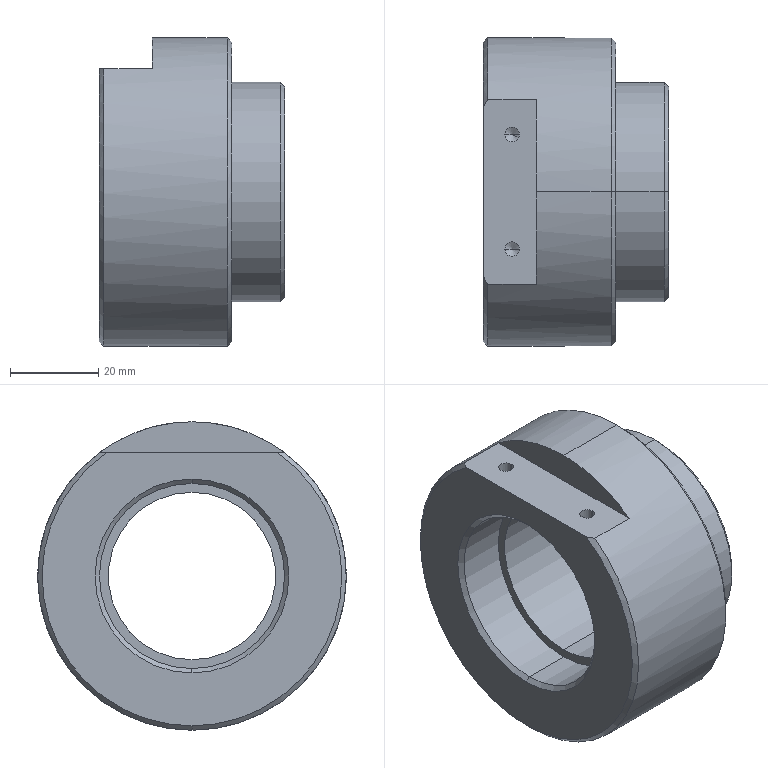Part | SolidWorks | features ICE 5, HoleWzd 2, Chamfer 1, CirPattern 1, Cut 1, Extrusion 1 | 1 solid | 51 faces | box 42 x 70 x 70 mm | volume 81911 mm3 | cone 22 | cylinder 22 | plane 7 | commonest cylinder face diameters 3.3 x12 42 x4 38 x2 49.9 x2 70 x2
STEP:
#1=CARTESIAN_POINT('',(0.,0.,-34.));
#2=VERTEX_POINT('',#1);
#3=CARTESIAN_POINT('',(0.,-19.287,28.));
#4=VERTEX_POINT('',#3);
#5=CARTESIAN_POINT('',(0.,0.,0.));
#6=DIRECTION('',(-1.,0.,0.));
#7=DIRECTION('',(0.,0.,-1.));
#8=AXIS2_PLACEMENT_3D('',#5,#6,#7);
#9=CIRCLE('',#8,34.);
#10=EDGE_CURVE('',#2,#4,#9,.T.);
#11=ORIENTED_EDGE('',*,*,#10,.F.);
#12=CARTESIAN_POINT('',(1.,0.,-35.));
#13=VERTEX_POINT('',#12);
#14=CARTESIAN_POINT('',(1.,0.,-35.));
#15=DIRECTION('',(0.7071,0.,-0.7071));
#16=VECTOR('',#15,1000.);
#17=LINE('',#14,#16);
#18=EDGE_CURVE('',#2,#13,#17,.T.);
#19=ORIENTED_EDGE('',*,*,#18,.T.);
#20=CARTESIAN_POINT('',(1.,-21.,28.));
#21=VERTEX_POINT('',#20);
#22=CARTESIAN_POINT('',(1.,0.,0.));
#23=DIRECTION('',(1.,0.,0.));
#24=DIRECTION('',(0.,0.,-1.));
#25=AXIS2_PLACEMENT_3D('',#22,#23,#24);
#26=CIRCLE('',#25,35.);
#27=EDGE_CURVE('',#21,#13,#26,.T.);
#28=ORIENTED_EDGE('',*,*,#27,.F.);
#29=CARTESIAN_POINT('',(0.,-19.287,28.));
#30=CARTESIAN_POINT('',(0.3262,-19.862,28.));
#31=CARTESIAN_POINT('',(0.6598,-20.433,28.));
#32=CARTESIAN_POINT('',(1.,-21.,28.));
#33=B_SPLINE_CURVE_WITH_KNOTS('',3,(#29,#30,#31,#32),.UNSPECIFIED.,.F.,.F.,(4,4),(0.,0.001983),.UNSPECIFIED.);
#34=EDGE_CURVE('',#4,#21,#33,.T.);
#35=ORIENTED_EDGE('',*,*,#34,.F.);
#36=EDGE_LOOP('',(#11,#19,#28,#35));
#37=FACE_OUTER_BOUND('',#36,.T.);
#38=CARTESIAN_POINT('',(1.,0.,0.));
#39=DIRECTION('',(1.,0.,0.));
#40=DIRECTION('',(0.,0.,-1.));
#41=AXIS2_PLACEMENT_3D('',#38,#39,#40);
#42=CONICAL_SURFACE('',#41,35.,0.7854);
#43=ADVANCED_FACE('',(#37),#42,.T.);
#44=CARTESIAN_POINT('',(30.,0.,-34.));
#45=VERTEX_POINT('',#44);
#46=CARTESIAN_POINT('',(30.,0.,34.));
#47=VERTEX_POINT('',#46);
#48=CARTESIAN_POINT('',(30.,0.,0.));
#49=DIRECTION('',(1.,0.,0.));
#50=DIRECTION('',(0.,0.,-1.));
#51=AXIS2_PLACEMENT_3D('',#48,#49,#50);
#52=CIRCLE('',#51,34.);
#53=EDGE_CURVE('',#45,#47,#52,.T.);
#54=ORIENTED_EDGE('',*,*,#53,.F.);
#55=CARTESIAN_POINT('',(29.,0.,-35.));
#56=VERTEX_POINT('',#55);
#57=CARTESIAN_POINT('',(30.,0.,-34.));
#58=DIRECTION('',(-0.7071,0.,-0.7071));
#59=VECTOR('',#58,1000.);
#60=LINE('',#57,#59);
#61=EDGE_CURVE('',#45,#56,#60,.T.);
#62=ORIENTED_EDGE('',*,*,#61,.T.);
#63=CARTESIAN_POINT('',(29.,0.,35.));
#64=VERTEX_POINT('',#63);
#65=CARTESIAN_POINT('',(29.,0.,0.));
#66=DIRECTION('',(-1.,0.,0.));
#67=DIRECTION('',(0.,0.,-1.));
#68=AXIS2_PLACEMENT_3D('',#65,#66,#67);
#69=CIRCLE('',#68,35.);
#70=EDGE_CURVE('',#64,#56,#69,.T.);
#71=ORIENTED_EDGE('',*,*,#70,.F.);
#72=CARTESIAN_POINT('',(30.,0.,34.));
#73=DIRECTION('',(-0.7071,0.,0.7071));
#74=VECTOR('',#73,1000.);
#75=LINE('',#72,#74);
#76=EDGE_CURVE('',#47,#64,#75,.T.);
#77=ORIENTED_EDGE('',*,*,#76,.F.);
#78=EDGE_LOOP('',(#54,#62,#71,#77));
#79=FACE_OUTER_BOUND('',#78,.T.);
#80=CARTESIAN_POINT('',(30.,0.,0.));
#81=DIRECTION('',(-1.,0.,0.));
#82=DIRECTION('',(0.,0.,1.));
#83=AXIS2_PLACEMENT_3D('',#80,#81,#82);
#84=CONICAL_SURFACE('',#83,34.,0.7854);
#85=ADVANCED_FACE('',(#79),#84,.T.);
#86=CARTESIAN_POINT('',(42.,0.,-23.95));
#87=VERTEX_POINT('',#86);
#88=CARTESIAN_POINT('',(42.,0.,23.95));
#89=VERTEX_POINT('',#88);
#90=CARTESIAN_POINT('',(42.,0.,0.));
#91=DIRECTION('',(1.,0.,0.));
#92=DIRECTION('',(0.,0.,-1.));
#93=AXIS2_PLACEMENT_3D('',#90,#91,#92);
#94=CIRCLE('',#93,23.95);
#95=EDGE_CURVE('',#87,#89,#94,.T.);
#96=ORIENTED_EDGE('',*,*,#95,.F.);
#97=CARTESIAN_POINT('',(41.,0.,-24.95));
#98=VERTEX_POINT('',#97);
#99=CARTESIAN_POINT('',(42.,0.,-23.95));
#100=DIRECTION('',(-0.7071,0.,-0.7071));
#101=VECTOR('',#100,1000.);
#102=LINE('',#99,#101);
#103=EDGE_CURVE('',#87,#98,#102,.T.);
#104=ORIENTED_EDGE('',*,*,#103,.T.);
#105=CARTESIAN_POINT('',(41.,0.,24.95));
#106=VERTEX_POINT('',#105);
#107=CARTESIAN_POINT('',(41.,0.,0.));
#108=DIRECTION('',(-1.,0.,0.));
#109=DIRECTION('',(0.,0.,-1.));
#110=AXIS2_PLACEMENT_3D('',#107,#108,#109);
#111=CIRCLE('',#110,24.95);
#112=EDGE_CURVE('',#106,#98,#111,.T.);
#113=ORIENTED_EDGE('',*,*,#112,.F.);
#114=CARTESIAN_POINT('',(42.,0.,23.95));
#115=DIRECTION('',(-0.7071,0.,0.7071));
#116=VECTOR('',#115,1000.);
#117=LINE('',#114,#116);
#118=EDGE_CURVE('',#89,#106,#117,.T.);
#119=ORIENTED_EDGE('',*,*,#118,.F.);
#120=EDGE_LOOP('',(#96,#104,#113,#119));
#121=FACE_OUTER_BOUND('',#120,.T.);
#122=CARTESIAN_POINT('',(42.,0.,0.));
#123=DIRECTION('',(-1.,0.,0.));
#124=DIRECTION('',(0.,0.,1.));
#125=AXIS2_PLACEMENT_3D('',#122,#123,#124);
#126=CONICAL_SURFACE('',#125,23.95,0.7854);
#127=ADVANCED_FACE('',(#121),#126,.T.);
#128=CARTESIAN_POINT('',(41.,0.,21.));
#129=VERTEX_POINT('',#128);
#130=CARTESIAN_POINT('',(41.,0.,-21.));
#131=VERTEX_POINT('',#130);
#132=CARTESIAN_POINT('',(41.,0.,0.));
#133=DIRECTION('',(1.,0.,0.));
#134=DIRECTION('',(0.,0.,-1.));
#135=AXIS2_PLACEMENT_3D('',#132,#133,#134);
#136=CIRCLE('',#135,21.);
#137=EDGE_CURVE('',#129,#131,#136,.T.);
#138=ORIENTED_EDGE('',*,*,#137,.F.);
#139=CARTESIAN_POINT('',(42.,0.,22.));
#140=VERTEX_POINT('',#139);
#141=CARTESIAN_POINT('',(41.,0.,21.));
#142=DIRECTION('',(0.7071,0.,0.7071));
#143=VECTOR('',#142,1000.);
#144=LINE('',#141,#143);
#145=EDGE_CURVE('',#129,#140,#144,.T.);
#146=ORIENTED_EDGE('',*,*,#145,.T.);
#147=CARTESIAN_POINT('',(42.,0.,-22.));
#148=VERTEX_POINT('',#147);
#149=CARTESIAN_POINT('',(42.,0.,0.));
#150=DIRECTION('',(-1.,0.,0.));
#151=DIRECTION('',(0.,0.,-1.));
#152=AXIS2_PLACEMENT_3D('',#149,#150,#151);
#153=CIRCLE('',#152,22.);
#154=EDGE_CURVE('',#148,#140,#153,.T.);
#155=ORIENTED_EDGE('',*,*,#154,.F.);
#156=CARTESIAN_POINT('',(41.,0.,-21.));
#157=DIRECTION('',(0.7071,0.,-0.7071));
#158=VECTOR('',#157,1000.);
#159=LINE('',#156,#158);
#160=EDGE_CURVE('',#131,#148,#159,.T.);
#161=ORIENTED_EDGE('',*,*,#160,.F.);
#162=EDGE_LOOP('',(#138,#146,#155,#161));
#163=FACE_OUTER_BOUND('',#162,.T.);
#164=CARTESIAN_POINT('',(41.,0.,0.));
#165=DIRECTION('',(1.,0.,0.));
#166=DIRECTION('',(0.,0.,-1.));
#167=AXIS2_PLACEMENT_3D('',#164,#165,#166);
#168=CONICAL_SURFACE('',#167,21.,0.7854);
#169=ADVANCED_FACE('',(#163),#168,.F.);
#170=CARTESIAN_POINT('',(1.,0.,-21.));
#171=VERTEX_POINT('',#170);
#172=CARTESIAN_POINT('',(1.,0.,21.));
#173=VERTEX_POINT('',#172);
#174=CARTESIAN_POINT('',(1.,0.,0.));
#175=DIRECTION('',(-1.,0.,0.));
#176=DIRECTION('',(0.,0.,-1.));
#177=AXIS2_PLACEMENT_3D('',#174,#175,#176);
#178=CIRCLE('',#177,21.);
#179=EDGE_CURVE('',#171,#173,#178,.T.);
#180=ORIENTED_EDGE('',*,*,#179,.F.);
#181=CARTESIAN_POINT('',(0.,0.,-22.));
#182=VERTEX_POINT('',#181);
#183=CARTESIAN_POINT('',(1.,0.,-21.));
#184=DIRECTION('',(-0.7071,0.,-0.7071));
#185=VECTOR('',#184,1000.);
#186=LINE('',#183,#185);
#187=EDGE_CURVE('',#171,#182,#186,.T.);
#188=ORIENTED_EDGE('',*,*,#187,.T.);
#189=CARTESIAN_POINT('',(0.,0.,22.));
#190=VERTEX_POINT('',#189);
#191=CARTESIAN_POINT('',(0.,0.,0.));
#192=DIRECTION('',(1.,0.,0.));
#193=DIRECTION('',(0.,0.,-1.));
#194=AXIS2_PLACEMENT_3D('',#191,#192,#193);
#195=CIRCLE('',#194,22.);
#196=EDGE_CURVE('',#190,#182,#195,.T.);
#197=ORIENTED_EDGE('',*,*,#196,.F.);
#198=CARTESIAN_POINT('',(1.,0.,21.));
#199=DIRECTION('',(-0.7071,0.,0.7071));
#200=VECTOR('',#199,1000.);
#201=LINE('',#198,#200);
#202=EDGE_CURVE('',#173,#190,#201,.T.);
#203=ORIENTED_EDGE('',*,*,#202,.F.);
#204=EDGE_LOOP('',(#180,#188,#197,#203));
#205=FACE_OUTER_BOUND('',#204,.T.);
#206=CARTESIAN_POINT('',(1.,0.,0.));
#207=DIRECTION('',(-1.,0.,0.));
#208=DIRECTION('',(0.,0.,1.));
#209=AXIS2_PLACEMENT_3D('',#206,#207,#208);
#210=CONICAL_SURFACE('',#209,21.,0.7854);
#211=ADVANCED_FACE('',(#205),#210,.F.);
#212=CARTESIAN_POINT('',(4.85,13.,17.9));
#213=VERTEX_POINT('',#212);
#214=CARTESIAN_POINT('',(8.15,13.,17.9));
#215=VERTEX_POINT('',#214);
#216=CARTESIAN_POINT('',(6.5,13.,17.9));
#217=DIRECTION('',(0.,0.,1.));
#218=DIRECTION('',(1.,0.,0.));
#219=AXIS2_PLACEMENT_3D('',#216,#217,#218);
#220=CIRCLE('',#219,1.65);
#221=EDGE_CURVE('',#213,#215,#220,.T.);
#222=ORIENTED_EDGE('',*,*,#221,.F.);
#223=CARTESIAN_POINT('',(4.85,13.,28.));
#224=VERTEX_POINT('',#223);
#225=CARTESIAN_POINT('',(4.85,13.,28.));
#226=DIRECTION('',(0.,0.,1.));
#227=VECTOR('',#226,1000.);
#228=LINE('',#225,#227);
#229=EDGE_CURVE('',#213,#224,#228,.T.);
#230=ORIENTED_EDGE('',*,*,#229,.T.);
#231=CARTESIAN_POINT('',(8.15,13.,28.));
#232=VERTEX_POINT('',#231);
#233=CARTESIAN_POINT('',(6.5,13.,28.));
#234=DIRECTION('',(0.,0.,1.));
#235=DIRECTION('',(1.,0.,0.));
#236=AXIS2_PLACEMENT_3D('',#233,#234,#235);
#237=CIRCLE('',#236,1.65);
#238=EDGE_CURVE('',#224,#232,#237,.T.);
#239=ORIENTED_EDGE('',*,*,#238,.T.);
#240=CARTESIAN_POINT('',(8.15,13.,28.));
#241=DIRECTION('',(0.,0.,1.));
#242=VECTOR('',#241,1000.);
#243=LINE('',#240,#242);
#244=EDGE_CURVE('',#215,#232,#243,.T.);
#245=ORIENTED_EDGE('',*,*,#244,.F.);
#246=EDGE_LOOP('',(#222,#230,#239,#245));
#247=FACE_OUTER_BOUND('',#246,.T.);
#248=CARTESIAN_POINT('',(6.5,13.,28.));
#249=DIRECTION('',(0.,0.,1.));
#250=DIRECTION('',(1.,0.,0.));
#251=AXIS2_PLACEMENT_3D('',#248,#249,#250);
#252=CYLINDRICAL_SURFACE('',#251,1.65);
#253=ADVANCED_FACE('',(#247),#252,.F.);
#254=CARTESIAN_POINT('',(6.5,13.,16.909));
#255=VERTEX_POINT('',#254);
#256=CARTESIAN_POINT('',(8.15,13.,17.9));
#257=DIRECTION('',(0.8572,0.,0.515));
#258=VECTOR('',#257,1000.);
#259=LINE('',#256,#258);
#260=EDGE_CURVE('',#255,#215,#259,.T.);
#261=ORIENTED_EDGE('',*,*,#260,.F.);
#262=CARTESIAN_POINT('',(4.85,13.,17.9));
#263=DIRECTION('',(-0.8572,0.,0.515));
#264=VECTOR('',#263,1000.);
#265=LINE('',#262,#264);
#266=EDGE_CURVE('',#255,#213,#265,.T.);
#267=ORIENTED_EDGE('',*,*,#266,.T.);
#268=ORIENTED_EDGE('',*,*,#221,.T.);
#269=EDGE_LOOP('',(#261,#267,#268));
#270=FACE_OUTER_BOUND('',#269,.T.);
#271=CARTESIAN_POINT('',(6.5,13.,17.9));
#272=DIRECTION('',(0.,0.,1.));
#273=DIRECTION('',(1.,0.,0.));
#274=AXIS2_PLACEMENT_3D('',#271,#272,#273);
#275=CONICAL_SURFACE('',#274,1.65,1.03);
#276=ADVANCED_FACE('',(#270),#275,.F.);
#277=CARTESIAN_POINT('',(4.85,-13.,17.9));
#278=VERTEX_POINT('',#277);
#279=CARTESIAN_POINT('',(8.15,-13.,17.9));
#280=VERTEX_POINT('',#279);
#281=CARTESIAN_POINT('',(6.5,-13.,17.9));
#282=DIRECTION('',(0.,0.,1.));
#283=DIRECTION('',(1.,0.,0.));
#284=AXIS2_PLACEMENT_3D('',#281,#282,#283);
#285=CIRCLE('',#284,1.65);
#286=EDGE_CURVE('',#278,#280,#285,.T.);
#287=ORIENTED_EDGE('',*,*,#286,.F.);
#288=CARTESIAN_POINT('',(4.85,-13.,28.));
#289=VERTEX_POINT('',#288);
#290=CARTESIAN_POINT('',(4.85,-13.,28.));
#291=DIRECTION('',(0.,0.,1.));
#292=VECTOR('',#291,1000.);
#293=LINE('',#290,#292);
#294=EDGE_CURVE('',#278,#289,#293,.T.);
#295=ORIENTED_EDGE('',*,*,#294,.T.);
#296=CARTESIAN_POINT('',(8.15,-13.,28.));
#297=VERTEX_POINT('',#296);
#298=CARTESIAN_POINT('',(6.5,-13.,28.));
#299=DIRECTION('',(0.,0.,1.));
#300=DIRECTION('',(1.,0.,0.));
#301=AXIS2_PLACEMENT_3D('',#298,#299,#300);
#302=CIRCLE('',#301,1.65);
#303=EDGE_CURVE('',#289,#297,#302,.T.);
#304=ORIENTED_EDGE('',*,*,#303,.T.);
#305=CARTESIAN_POINT('',(8.15,-13.,28.));
#306=DIRECTION('',(0.,0.,1.));
#307=VECTOR('',#306,1000.);
#308=LINE('',#305,#307);
#309=EDGE_CURVE('',#280,#297,#308,.T.);
#310=ORIENTED_EDGE('',*,*,#309,.F.);
#311=EDGE_LOOP('',(#287,#295,#304,#310));
#312=FACE_OUTER_BOUND('',#311,.T.);
#313=CARTESIAN_POINT('',(6.5,-13.,28.));
#314=DIRECTION('',(0.,0.,1.));
#315=DIRECTION('',(1.,0.,0.));
#316=AXIS2_PLACEMENT_3D('',#313,#314,#315);
#317=CYLINDRICAL_SURFACE('',#316,1.65);
#318=ADVANCED_FACE('',(#312),#317,.F.);
#319=CARTESIAN_POINT('',(6.5,-13.,16.909));
#320=VERTEX_POINT('',#319);
#321=CARTESIAN_POINT('',(8.15,-13.,17.9));
#322=DIRECTION('',(0.8572,0.,0.515));
#323=VECTOR('',#322,1000.);
#324=LINE('',#321,#323);
#325=EDGE_CURVE('',#320,#280,#324,.T.);
#326=ORIENTED_EDGE('',*,*,#325,.F.);
#327=CARTESIAN_POINT('',(4.85,-13.,17.9));
#328=DIRECTION('',(-0.8572,0.,0.515));
#329=VECTOR('',#328,1000.);
#330=LINE('',#327,#329);
#331=EDGE_CURVE('',#320,#278,#330,.T.);
#332=ORIENTED_EDGE('',*,*,#331,.T.);
#333=ORIENTED_EDGE('',*,*,#286,.T.);
#334=EDGE_LOOP('',(#326,#332,#333));
#335=FACE_OUTER_BOUND('',#334,.T.);
#336=CARTESIAN_POINT('',(6.5,-13.,17.9));
#337=DIRECTION('',(0.,0.,1.));
#338=DIRECTION('',(1.,0.,0.));
#339=AXIS2_PLACEMENT_3D('',#336,#337,#338);
#340=CONICAL_SURFACE('',#339,1.65,1.03);
#341=ADVANCED_FACE('',(#335),#340,.F.);
#342=CARTESIAN_POINT('',(19.9,30.,1.65));
#343=VERTEX_POINT('',#342);
#344=CARTESIAN_POINT('',(19.9,30.,-1.65));
#345=VERTEX_POINT('',#344);
#346=CARTESIAN_POINT('',(19.9,30.,0.));
#347=DIRECTION('',(1.,0.,0.));
#348=DIRECTION('',(0.,0.,-1.));
#349=AXIS2_PLACEMENT_3D('',#346,#347,#348);
#350=CIRCLE('',#349,1.65);
#351=EDGE_CURVE('',#343,#345,#350,.T.);
#352=ORIENTED_EDGE('',*,*,#351,.F.);
#353=CARTESIAN_POINT('',(30.,30.,1.65));
#354=VERTEX_POINT('',#353);
#355=CARTESIAN_POINT('',(30.,30.,1.65));
#356=DIRECTION('',(1.,0.,0.));
#357=VECTOR('',#356,1000.);
#358=LINE('',#355,#357);
#359=EDGE_CURVE('',#343,#354,#358,.T.);
#360=ORIENTED_EDGE('',*,*,#359,.T.);
#361=CARTESIAN_POINT('',(30.,30.,-1.65));
#362=VERTEX_POINT('',#361);
#363=CARTESIAN_POINT('',(30.,30.,0.));
#364=DIRECTION('',(1.,0.,0.));
#365=DIRECTION('',(0.,0.,-1.));
#366=AXIS2_PLACEMENT_3D('',#363,#364,#365);
#367=CIRCLE('',#366,1.65);
#368=EDGE_CURVE('',#354,#362,#367,.T.);
#369=ORIENTED_EDGE('',*,*,#368,.T.);
#370=CARTESIAN_POINT('',(30.,30.,-1.65));
#371=DIRECTION('',(1.,0.,0.));
#372=VECTOR('',#371,1000.);
#373=LINE('',#370,#372);
#374=EDGE_CURVE('',#345,#362,#373,.T.);
#375=ORIENTED_EDGE('',*,*,#374,.F.);
#376=EDGE_LOOP('',(#352,#360,#369,#375));
#377=FACE_OUTER_BOUND('',#376,.T.);
#378=CARTESIAN_POINT('',(30.,30.,0.));
#379=DIRECTION('',(1.,0.,0.));
#380=DIRECTION('',(0.,0.,-1.));
#381=AXIS2_PLACEMENT_3D('',#378,#379,#380);
#382=CYLINDRICAL_SURFACE('',#381,1.65);
#383=ADVANCED_FACE('',(#377),#382,.F.);
#384=CARTESIAN_POINT('',(18.909,30.,0.));
#385=VERTEX_POINT('',#384);
#386=CARTESIAN_POINT('',(19.9,30.,-1.65));
#387=DIRECTION('',(0.515,0.,-0.8572));
#388=VECTOR('',#387,1000.);
#389=LINE('',#386,#388);
#390=EDGE_CURVE('',#385,#345,#389,.T.);
#391=ORIENTED_EDGE('',*,*,#390,.F.);
#392=CARTESIAN_POINT('',(19.9,30.,1.65));
#393=DIRECTION('',(0.515,0.,0.8572));
#394=VECTOR('',#393,1000.);
#395=LINE('',#392,#394);
#396=EDGE_CURVE('',#385,#343,#395,.T.);
#397=ORIENTED_EDGE('',*,*,#396,.T.);
#398=ORIENTED_EDGE('',*,*,#351,.T.);
#399=EDGE_LOOP('',(#391,#397,#398));
#400=FACE_OUTER_BOUND('',#399,.T.);
#401=CARTESIAN_POINT('',(19.9,30.,0.));
#402=DIRECTION('',(1.,0.,0.));
#403=DIRECTION('',(0.,0.,-1.));
#404=AXIS2_PLACEMENT_3D('',#401,#402,#403);
#405=CONICAL_SURFACE('',#404,1.65,1.03);
#406=ADVANCED_FACE('',(#400),#405,.F.);
#407=CARTESIAN_POINT('',(19.9,0.,31.65));
#408=VERTEX_POINT('',#407);
#409=CARTESIAN_POINT('',(19.9,0.,28.35));
#410=VERTEX_POINT('',#409);
#411=CARTESIAN_POINT('',(19.9,0.,30.));
#412=DIRECTION('',(1.,0.,0.));
#413=DIRECTION('',(0.,0.,-1.));
#414=AXIS2_PLACEMENT_3D('',#411,#412,#413);
#415=CIRCLE('',#414,1.65);
#416=EDGE_CURVE('',#408,#410,#415,.T.);
#417=ORIENTED_EDGE('',*,*,#416,.F.);
#418=CARTESIAN_POINT('',(30.,0.,31.65));
#419=VERTEX_POINT('',#418);
#420=CARTESIAN_POINT('',(30.,0.,31.65));
#421=DIRECTION('',(1.,0.,0.));
#422=VECTOR('',#421,1000.);
#423=LINE('',#420,#422);
#424=EDGE_CURVE('',#408,#419,#423,.T.);
#425=ORIENTED_EDGE('',*,*,#424,.T.);
#426=CARTESIAN_POINT('',(30.,0.,28.35));
#427=VERTEX_POINT('',#426);
#428=CARTESIAN_POINT('',(30.,0.,30.));
#429=DIRECTION('',(1.,0.,0.));
#430=DIRECTION('',(0.,0.,-1.));
#431=AXIS2_PLACEMENT_3D('',#428,#429,#430);
#432=CIRCLE('',#431,1.65);
#433=EDGE_CURVE('',#419,#427,#432,.T.);
#434=ORIENTED_EDGE('',*,*,#433,.T.);
#435=CARTESIAN_POINT('',(30.,0.,28.35));
#436=DIRECTION('',(1.,0.,0.));
#437=VECTOR('',#436,1000.);
#438=LINE('',#435,#437);
#439=EDGE_CURVE('',#410,#427,#438,.T.);
#440=ORIENTED_EDGE('',*,*,#439,.F.);
#441=EDGE_LOOP('',(#417,#425,#434,#440));
#442=FACE_OUTER_BOUND('',#441,.T.);
#443=CARTESIAN_POINT('',(30.,0.,30.));
#444=DIRECTION('',(1.,0.,0.));
#445=DIRECTION('',(0.,0.,-1.));
#446=AXIS2_PLACEMENT_3D('',#443,#444,#445);
#447=CYLINDRICAL_SURFACE('',#446,1.65);
#448=ADVANCED_FACE('',(#442),#447,.F.);
#449=CARTESIAN_POINT('',(18.909,0.,30.));
#450=VERTEX_POINT('',#449);
#451=CARTESIAN_POINT('',(19.9,0.,28.35));
#452=DIRECTION('',(0.515,0.,-0.8572));
#453=VECTOR('',#452,1000.);
#454=LINE('',#451,#453);
#455=EDGE_CURVE('',#450,#410,#454,.T.);
#456=ORIENTED_EDGE('',*,*,#455,.F.);
#457=CARTESIAN_POINT('',(19.9,0.,31.65));
#458=DIRECTION('',(0.515,0.,0.8572));
#459=VECTOR('',#458,1000.);
#460=LINE('',#457,#459);
#461=EDGE_CURVE('',#450,#408,#460,.T.);
#462=ORIENTED_EDGE('',*,*,#461,.T.);
#463=ORIENTED_EDGE('',*,*,#416,.T.);
#464=EDGE_LOOP('',(#456,#462,#463));
#465=FACE_OUTER_BOUND('',#464,.T.);
#466=CARTESIAN_POINT('',(19.9,0.,30.));
#467=DIRECTION('',(1.,0.,0.));
#468=DIRECTION('',(0.,0.,-1.));
#469=AXIS2_PLACEMENT_3D('',#466,#467,#468);
#470=CONICAL_SURFACE('',#469,1.65,1.03);
#471=ADVANCED_FACE('',(#465),#470,.F.);
#472=CARTESIAN_POINT('',(19.9,-30.,1.65));
#473=VERTEX_POINT('',#472);
#474=CARTESIAN_POINT('',(19.9,-30.,-1.65));
#475=VERTEX_POINT('',#474);
#476=CARTESIAN_POINT('',(19.9,-30.,0.));
#477=DIRECTION('',(1.,0.,0.));
#478=DIRECTION('',(0.,0.,-1.));
#479=AXIS2_PLACEMENT_3D('',#476,#477,#478);
#480=CIRCLE('',#479,1.65);
#481=EDGE_CURVE('',#473,#475,#480,.T.);
#482=ORIENTED_EDGE('',*,*,#481,.F.);
#483=CARTESIAN_POINT('',(30.,-30.,1.65));
#484=VERTEX_POINT('',#483);
#485=CARTESIAN_POINT('',(30.,-30.,1.65));
#486=DIRECTION('',(1.,0.,0.));
#487=VECTOR('',#486,1000.);
#488=LINE('',#485,#487);
#489=EDGE_CURVE('',#473,#484,#488,.T.);
#490=ORIENTED_EDGE('',*,*,#489,.T.);
#491=CARTESIAN_POINT('',(30.,-30.,-1.65));
#492=VERTEX_POINT('',#491);
#493=CARTESIAN_POINT('',(30.,-30.,0.));
#494=DIRECTION('',(1.,0.,0.));
#495=DIRECTION('',(0.,0.,-1.));
#496=AXIS2_PLACEMENT_3D('',#493,#494,#495);
#497=CIRCLE('',#496,1.65);
#498=EDGE_CURVE('',#484,#492,#497,.T.);
#499=ORIENTED_EDGE('',*,*,#498,.T.);
#500=CARTESIAN_POINT('',(30.,-30.,-1.65));
#501=DIRECTION('',(1.,0.,0.));
#502=VECTOR('',#501,1000.);
#503=LINE('',#500,#502);
#504=EDGE_CURVE('',#475,#492,#503,.T.);
#505=ORIENTED_EDGE('',*,*,#504,.F.);
#506=EDGE_LOOP('',(#482,#490,#499,#505));
#507=FACE_OUTER_BOUND('',#506,.T.);
#508=CARTESIAN_POINT('',(30.,-30.,0.));
#509=DIRECTION('',(1.,0.,0.));
#510=DIRECTION('',(0.,0.,-1.));
#511=AXIS2_PLACEMENT_3D('',#508,#509,#510);
#512=CYLINDRICAL_SURFACE('',#511,1.65);
#513=ADVANCED_FACE('',(#507),#512,.F.);
#514=CARTESIAN_POINT('',(18.909,-30.,0.));
#515=VERTEX_POINT('',#514);
#516=CARTESIAN_POINT('',(19.9,-30.,-1.65));
#517=DIRECTION('',(0.515,0.,-0.8572));
#518=VECTOR('',#517,1000.);
#519=LINE('',#516,#518);
#520=EDGE_CURVE('',#515,#475,#519,.T.);
#521=ORIENTED_EDGE('',*,*,#520,.F.);
#522=CARTESIAN_POINT('',(19.9,-30.,1.65));
#523=DIRECTION('',(0.515,0.,0.8572));
#524=VECTOR('',#523,1000.);
#525=LINE('',#522,#524);
#526=EDGE_CURVE('',#515,#473,#525,.T.);
#527=ORIENTED_EDGE('',*,*,#526,.T.);
#528=ORIENTED_EDGE('',*,*,#481,.T.);
#529=EDGE_LOOP('',(#521,#527,#528));
#530=FACE_OUTER_BOUND('',#529,.T.);
#531=CARTESIAN_POINT('',(19.9,-30.,0.));
#532=DIRECTION('',(1.,0.,0.));
#533=DIRECTION('',(0.,0.,-1.));
#534=AXIS2_PLACEMENT_3D('',#531,#532,#533);
#535=CONICAL_SURFACE('',#534,1.65,1.03);
#536=ADVANCED_FACE('',(#530),#535,.F.);
#537=CARTESIAN_POINT('',(19.9,0.,-28.35));
#538=VERTEX_POINT('',#537);
#539=CARTESIAN_POINT('',(19.9,0.,-31.65));
#540=VERTEX_POINT('',#539);
#541=CARTESIAN_POINT('',(19.9,0.,-30.));
#542=DIRECTION('',(1.,0.,0.));
#543=DIRECTION('',(0.,0.,-1.));
#544=AXIS2_PLACEMENT_3D('',#541,#542,#543);
#545=CIRCLE('',#544,1.65);
#546=EDGE_CURVE('',#538,#540,#545,.T.);
#547=ORIENTED_EDGE('',*,*,#546,.F.);
#548=CARTESIAN_POINT('',(30.,0.,-28.35));
#549=VERTEX_POINT('',#548);
#550=CARTESIAN_POINT('',(30.,0.,-28.35));
#551=DIRECTION('',(1.,0.,0.));
#552=VECTOR('',#551,1000.);
#553=LINE('',#550,#552);
#554=EDGE_CURVE('',#538,#549,#553,.T.);
#555=ORIENTED_EDGE('',*,*,#554,.T.);
#556=CARTESIAN_POINT('',(30.,0.,-31.65));
#557=VERTEX_POINT('',#556);
#558=CARTESIAN_POINT('',(30.,0.,-30.));
#559=DIRECTION('',(1.,0.,0.));
#560=DIRECTION('',(0.,0.,-1.));
#561=AXIS2_PLACEMENT_3D('',#558,#559,#560);
#562=CIRCLE('',#561,1.65);
#563=EDGE_CURVE('',#549,#557,#562,.T.);
#564=ORIENTED_EDGE('',*,*,#563,.T.);
#565=CARTESIAN_POINT('',(30.,0.,-31.65));
#566=DIRECTION('',(1.,0.,0.));
#567=VECTOR('',#566,1000.);
#568=LINE('',#565,#567);
#569=EDGE_CURVE('',#540,#557,#568,.T.);
#570=ORIENTED_EDGE('',*,*,#569,.F.);
#571=EDGE_LOOP('',(#547,#555,#564,#570));
#572=FACE_OUTER_BOUND('',#571,.T.);
#573=CARTESIAN_POINT('',(30.,0.,-30.));
#574=DIRECTION('',(1.,0.,0.));
#575=DIRECTION('',(0.,0.,-1.));
#576=AXIS2_PLACEMENT_3D('',#573,#574,#575);
#577=CYLINDRICAL_SURFACE('',#576,1.65);
#578=ADVANCED_FACE('',(#572),#577,.F.);
#579=CARTESIAN_POINT('',(18.909,0.,-30.));
#580=VERTEX_POINT('',#579);
#581=CARTESIAN_POINT('',(19.9,0.,-31.65));
#582=DIRECTION('',(0.515,0.,-0.8572));
#583=VECTOR('',#582,1000.);
#584=LINE('',#581,#583);
#585=EDGE_CURVE('',#580,#540,#584,.T.);
#586=ORIENTED_EDGE('',*,*,#585,.F.);
#587=CARTESIAN_POINT('',(19.9,0.,-28.35));
#588=DIRECTION('',(0.515,0.,0.8572));
#589=VECTOR('',#588,1000.);
#590=LINE('',#587,#589);
#591=EDGE_CURVE('',#580,#538,#590,.T.);
#592=ORIENTED_EDGE('',*,*,#591,.T.);
#593=ORIENTED_EDGE('',*,*,#546,.T.);
#594=EDGE_LOOP('',(#586,#592,#593));
#595=FACE_OUTER_BOUND('',#594,.T.);
#596=CARTESIAN_POINT('',(19.9,0.,-30.));
#597=DIRECTION('',(1.,0.,0.));
#598=DIRECTION('',(0.,0.,-1.));
#599=AXIS2_PLACEMENT_3D('',#596,#597,#598);
#600=CONICAL_SURFACE('',#599,1.65,1.03);
#601=ADVANCED_FACE('',(#595),#600,.F.);
#602=ORIENTED_EDGE('',*,*,#137,.T.);
#603=CARTESIAN_POINT('',(30.,0.,-21.));
#604=VERTEX_POINT('',#603);
#605=CARTESIAN_POINT('',(58.,0.,-21.));
#606=DIRECTION('',(-1.,0.,0.));
#607=VECTOR('',#606,1000.);
#608=LINE('',#605,#607);
#609=EDGE_CURVE('',#131,#604,#608,.T.);
#610=ORIENTED_EDGE('',*,*,#609,.T.);
#611=CARTESIAN_POINT('',(30.,0.,21.));
#612=VERTEX_POINT('',#611);
#613=CARTESIAN_POINT('',(30.,0.,0.));
#614=DIRECTION('',(-1.,0.,0.));
#615=DIRECTION('',(0.,0.,1.));
#616=AXIS2_PLACEMENT_3D('',#613,#614,#615);
#617=CIRCLE('',#616,21.);
#618=EDGE_CURVE('',#604,#612,#617,.T.);
#619=ORIENTED_EDGE('',*,*,#618,.T.);
#620=CARTESIAN_POINT('',(58.,0.,21.));
#621=DIRECTION('',(-1.,0.,0.));
#622=VECTOR('',#621,1000.);
#623=LINE('',#620,#622);
#624=EDGE_CURVE('',#129,#612,#623,.T.);
#625=ORIENTED_EDGE('',*,*,#624,.F.);
#626=EDGE_LOOP('',(#602,#610,#619,#625));
#627=FACE_OUTER_BOUND('',#626,.T.);
#628=CARTESIAN_POINT('',(58.,0.,0.));
#629=DIRECTION('',(-1.,0.,0.));
#630=DIRECTION('',(0.,0.,1.));
#631=AXIS2_PLACEMENT_3D('',#628,#629,#630);
#632=CYLINDRICAL_SURFACE('',#631,21.);
#633=ADVANCED_FACE('',(#627),#632,.F.);
#634=CARTESIAN_POINT('',(30.,0.,19.));
#635=VERTEX_POINT('',#634);
#636=CARTESIAN_POINT('',(30.,0.,-19.));
#637=VERTEX_POINT('',#636);
#638=CARTESIAN_POINT('',(30.,0.,0.));
#639=DIRECTION('',(1.,0.,0.));
#640=DIRECTION('',(0.,0.,1.));
#641=AXIS2_PLACEMENT_3D('',#638,#639,#640);
#642=CIRCLE('',#641,19.);
#643=EDGE_CURVE('',#635,#637,#642,.T.);
#644=ORIENTED_EDGE('',*,*,#643,.T.);
#645=CARTESIAN_POINT('',(12.,0.,-19.));
#646=VERTEX_POINT('',#645);
#647=CARTESIAN_POINT('',(30.,0.,-19.));
#648=DIRECTION('',(-1.,0.,0.));
#649=VECTOR('',#648,1000.);
#650=LINE('',#647,#649);
#651=EDGE_CURVE('',#637,#646,#650,.T.);
#652=ORIENTED_EDGE('',*,*,#651,.T.);
#653=CARTESIAN_POINT('',(12.,0.,19.));
#654=VERTEX_POINT('',#653);
#655=CARTESIAN_POINT('',(12.,0.,0.));
#656=DIRECTION('',(-1.,0.,0.));
#657=DIRECTION('',(0.,0.,1.));
#658=AXIS2_PLACEMENT_3D('',#655,#656,#657);
#659=CIRCLE('',#658,19.);
#660=EDGE_CURVE('',#646,#654,#659,.T.);
#661=ORIENTED_EDGE('',*,*,#660,.T.);
#662=CARTESIAN_POINT('',(30.,0.,19.));
#663=DIRECTION('',(-1.,0.,0.));
#664=VECTOR('',#663,1000.);
#665=LINE('',#662,#664);
#666=EDGE_CURVE('',#635,#654,#665,.T.);
#667=ORIENTED_EDGE('',*,*,#666,.F.);
#668=EDGE_LOOP('',(#644,#652,#661,#667));
#669=FACE_OUTER_BOUND('',#668,.T.);
#670=CARTESIAN_POINT('',(30.,0.,0.));
#671=DIRECTION('',(-1.,0.,0.));
#672=DIRECTION('',(0.,0.,1.));
#673=AXIS2_PLACEMENT_3D('',#670,#671,#672);
#674=CYLINDRICAL_SURFACE('',#673,19.);
#675=ADVANCED_FACE('',(#669),#674,.F.);
#676=CARTESIAN_POINT('',(12.,0.,-21.));
#677=VERTEX_POINT('',#676);
#678=CARTESIAN_POINT('',(12.,0.,21.));
#679=VERTEX_POINT('',#678);
#680=CARTESIAN_POINT('',(12.,0.,0.));
#681=DIRECTION('',(-1.,0.,0.));
#682=DIRECTION('',(0.,0.,1.));
#683=AXIS2_PLACEMENT_3D('',#680,#681,#682);
#684=CIRCLE('',#683,21.);
#685=EDGE_CURVE('',#677,#679,#684,.T.);
#686=ORIENTED_EDGE('',*,*,#685,.F.);
#687=CARTESIAN_POINT('',(12.,0.,-21.));
#688=DIRECTION('',(-1.,0.,0.));
#689=VECTOR('',#688,1000.);
#690=LINE('',#687,#689);
#691=EDGE_CURVE('',#677,#171,#690,.T.);
#692=ORIENTED_EDGE('',*,*,#691,.T.);
#693=ORIENTED_EDGE('',*,*,#179,.T.);
#694=CARTESIAN_POINT('',(12.,0.,21.));
#695=DIRECTION('',(-1.,0.,0.));
#696=VECTOR('',#695,1000.);
#697=LINE('',#694,#696);
#698=EDGE_CURVE('',#679,#173,#697,.T.);
#699=ORIENTED_EDGE('',*,*,#698,.F.);
#700=EDGE_LOOP('',(#686,#692,#693,#699));
#701=FACE_OUTER_BOUND('',#700,.T.);
#702=CARTESIAN_POINT('',(12.,0.,0.));
#703=DIRECTION('',(-1.,0.,0.));
#704=DIRECTION('',(0.,0.,1.));
#705=AXIS2_PLACEMENT_3D('',#702,#703,#704);
#706=CYLINDRICAL_SURFACE('',#705,21.);
#707=ADVANCED_FACE('',(#701),#706,.F.);
#708=ORIENTED_EDGE('',*,*,#112,.T.);
#709=CARTESIAN_POINT('',(30.,0.,-24.95));
#710=VERTEX_POINT('',#709);
#711=CARTESIAN_POINT('',(42.,0.,-24.95));
#712=DIRECTION('',(-1.,0.,0.));
#713=VECTOR('',#712,1000.);
#714=LINE('',#711,#713);
#715=EDGE_CURVE('',#98,#710,#714,.T.);
#716=ORIENTED_EDGE('',*,*,#715,.T.);
#717=CARTESIAN_POINT('',(30.,0.,24.95));
#718=VERTEX_POINT('',#717);
#719=CARTESIAN_POINT('',(30.,0.,0.));
#720=DIRECTION('',(1.,0.,0.));
#721=DIRECTION('',(0.,0.,-1.));
#722=AXIS2_PLACEMENT_3D('',#719,#720,#721);
#723=CIRCLE('',#722,24.95);
#724=EDGE_CURVE('',#710,#718,#723,.T.);
#725=ORIENTED_EDGE('',*,*,#724,.T.);
#726=CARTESIAN_POINT('',(42.,0.,24.95));
#727=DIRECTION('',(-1.,0.,0.));
#728=VECTOR('',#727,1000.);
#729=LINE('',#726,#728);
#730=EDGE_CURVE('',#106,#718,#729,.T.);
#731=ORIENTED_EDGE('',*,*,#730,.F.);
#732=EDGE_LOOP('',(#708,#716,#725,#731));
#733=FACE_OUTER_BOUND('',#732,.T.);
#734=CARTESIAN_POINT('',(42.,0.,0.));
#735=DIRECTION('',(-1.,0.,0.));
#736=DIRECTION('',(0.,0.,1.));
#737=AXIS2_PLACEMENT_3D('',#734,#735,#736);
#738=CYLINDRICAL_SURFACE('',#737,24.95);
#739=ADVANCED_FACE('',(#733),#738,.T.);
#740=ORIENTED_EDGE('',*,*,#70,.T.);
#741=CARTESIAN_POINT('',(20.,0.,-35.));
#742=DIRECTION('',(-1.,0.,0.));
#743=VECTOR('',#742,1000.);
#744=LINE('',#741,#743);
#745=EDGE_CURVE('',#56,#13,#744,.T.);
#746=ORIENTED_EDGE('',*,*,#745,.T.);
#747=CARTESIAN_POINT('',(1.,21.,28.));
#748=VERTEX_POINT('',#747);
#749=CARTESIAN_POINT('',(1.,0.,0.));
#750=DIRECTION('',(1.,0.,0.));
#751=DIRECTION('',(0.,0.,-1.));
#752=AXIS2_PLACEMENT_3D('',#749,#750,#751);
#753=CIRCLE('',#752,35.);
#754=EDGE_CURVE('',#13,#748,#753,.T.);
#755=ORIENTED_EDGE('',*,*,#754,.T.);
#756=CARTESIAN_POINT('',(12.,21.,28.));
#757=VERTEX_POINT('',#756);
#758=CARTESIAN_POINT('',(20.,21.,28.));
#759=DIRECTION('',(1.,0.,0.));
#760=VECTOR('',#759,1000.);
#761=LINE('',#758,#760);
#762=EDGE_CURVE('',#748,#757,#761,.T.);
#763=ORIENTED_EDGE('',*,*,#762,.T.);
#764=CARTESIAN_POINT('',(12.,0.,35.));
#765=VERTEX_POINT('',#764);
#766=CARTESIAN_POINT('',(12.,0.,0.));
#767=DIRECTION('',(-1.,0.,0.));
#768=DIRECTION('',(0.,0.,1.));
#769=AXIS2_PLACEMENT_3D('',#766,#767,#768);
#770=CIRCLE('',#769,35.);
#771=EDGE_CURVE('',#765,#757,#770,.T.);
#772=ORIENTED_EDGE('',*,*,#771,.F.);
#773=CARTESIAN_POINT('',(20.,0.,35.));
#774=DIRECTION('',(-1.,0.,0.));
#775=VECTOR('',#774,1000.);
#776=LINE('',#773,#775);
#777=EDGE_CURVE('',#64,#765,#776,.T.);
#778=ORIENTED_EDGE('',*,*,#777,.F.);
#779=EDGE_LOOP('',(#740,#746,#755,#763,#772,#778));
#780=FACE_OUTER_BOUND('',#779,.T.);
#781=CARTESIAN_POINT('',(20.,0.,0.));
#782=DIRECTION('',(-1.,0.,0.));
#783=DIRECTION('',(0.,0.,1.));
#784=AXIS2_PLACEMENT_3D('',#781,#782,#783);
#785=CYLINDRICAL_SURFACE('',#784,35.);
#786=ADVANCED_FACE('',(#780),#785,.T.);
#787=CARTESIAN_POINT('',(30.,0.,0.));
#788=DIRECTION('',(1.,0.,0.));
#789=DIRECTION('',(0.,0.,-1.));
#790=AXIS2_PLACEMENT_3D('',#787,#788,#789);
#791=CIRCLE('',#790,34.);
#792=EDGE_CURVE('',#47,#45,#791,.T.);
#793=ORIENTED_EDGE('',*,*,#792,.T.);
#794=ORIENTED_EDGE('',*,*,#53,.T.);
#795=EDGE_LOOP('',(#793,#794));
#796=FACE_OUTER_BOUND('',#795,.T.);
#797=CARTESIAN_POINT('',(30.,30.,0.));
#798=DIRECTION('',(1.,0.,0.));
#799=DIRECTION('',(0.,0.,-1.));
#800=AXIS2_PLACEMENT_3D('',#797,#798,#799);
#801=CIRCLE('',#800,1.65);
#802=EDGE_CURVE('',#362,#354,#801,.T.);
#803=ORIENTED_EDGE('',*,*,#802,.F.);
#804=ORIENTED_EDGE('',*,*,#368,.F.);
#805=EDGE_LOOP('',(#803,#804));
#806=FACE_BOUND('',#805,.T.);
#807=CARTESIAN_POINT('',(30.,0.,30.));
#808=DIRECTION('',(1.,0.,0.));
#809=DIRECTION('',(0.,0.,-1.));
#810=AXIS2_PLACEMENT_3D('',#807,#808,#809);
#811=CIRCLE('',#810,1.65);
#812=EDGE_CURVE('',#427,#419,#811,.T.);
#813=ORIENTED_EDGE('',*,*,#812,.F.);
#814=ORIENTED_EDGE('',*,*,#433,.F.);
#815=EDGE_LOOP('',(#813,#814));
#816=FACE_BOUND('',#815,.T.);
#817=CARTESIAN_POINT('',(30.,-30.,0.));
#818=DIRECTION('',(1.,0.,0.));
#819=DIRECTION('',(0.,0.,-1.));
#820=AXIS2_PLACEMENT_3D('',#817,#818,#819);
#821=CIRCLE('',#820,1.65);
#822=EDGE_CURVE('',#492,#484,#821,.T.);
#823=ORIENTED_EDGE('',*,*,#822,.F.);
#824=ORIENTED_EDGE('',*,*,#498,.F.);
#825=EDGE_LOOP('',(#823,#824));
#826=FACE_BOUND('',#825,.T.);
#827=CARTESIAN_POINT('',(30.,0.,-30.));
#828=DIRECTION('',(1.,0.,0.));
#829=DIRECTION('',(0.,0.,-1.));
#830=AXIS2_PLACEMENT_3D('',#827,#828,#829);
#831=CIRCLE('',#830,1.65);
#832=EDGE_CURVE('',#557,#549,#831,.T.);
#833=ORIENTED_EDGE('',*,*,#832,.F.);
#834=ORIENTED_EDGE('',*,*,#563,.F.);
#835=EDGE_LOOP('',(#833,#834));
#836=FACE_BOUND('',#835,.T.);
#837=CARTESIAN_POINT('',(30.,0.,0.));
#838=DIRECTION('',(1.,0.,0.));
#839=DIRECTION('',(0.,0.,-1.));
#840=AXIS2_PLACEMENT_3D('',#837,#838,#839);
#841=CIRCLE('',#840,24.95);
#842=EDGE_CURVE('',#718,#710,#841,.T.);
#843=ORIENTED_EDGE('',*,*,#842,.F.);
#844=ORIENTED_EDGE('',*,*,#724,.F.);
#845=EDGE_LOOP('',(#843,#844));
#846=FACE_BOUND('',#845,.T.);
#847=CARTESIAN_POINT('',(30.,0.,0.));
#848=DIRECTION('',(1.,0.,0.));
#849=DIRECTION('',(0.,0.,-1.));
#850=AXIS2_PLACEMENT_3D('',#847,#848,#849);
#851=PLANE('',#850);
#852=ADVANCED_FACE('',(#796,#806,#816,#826,#836,#846),#851,.T.);
#853=ORIENTED_EDGE('',*,*,#745,.F.);
#854=CARTESIAN_POINT('',(29.,0.,0.));
#855=DIRECTION('',(-1.,0.,0.));
#856=DIRECTION('',(0.,0.,-1.));
#857=AXIS2_PLACEMENT_3D('',#854,#855,#856);
#858=CIRCLE('',#857,35.);
#859=EDGE_CURVE('',#56,#64,#858,.T.);
#860=ORIENTED_EDGE('',*,*,#859,.T.);
#861=ORIENTED_EDGE('',*,*,#777,.T.);
#862=CARTESIAN_POINT('',(12.,-21.,28.));
#863=VERTEX_POINT('',#862);
#864=CARTESIAN_POINT('',(12.,0.,0.));
#865=DIRECTION('',(-1.,0.,0.));
#866=DIRECTION('',(0.,0.,1.));
#867=AXIS2_PLACEMENT_3D('',#864,#865,#866);
#868=CIRCLE('',#867,35.);
#869=EDGE_CURVE('',#863,#765,#868,.T.);
#870=ORIENTED_EDGE('',*,*,#869,.F.);
#871=CARTESIAN_POINT('',(20.,-21.,28.));
#872=DIRECTION('',(-1.,0.,0.));
#873=VECTOR('',#872,1000.);
#874=LINE('',#871,#873);
#875=EDGE_CURVE('',#863,#21,#874,.T.);
#876=ORIENTED_EDGE('',*,*,#875,.T.);
#877=ORIENTED_EDGE('',*,*,#27,.T.);
#878=EDGE_LOOP('',(#853,#860,#861,#870,#876,#877));
#879=FACE_OUTER_BOUND('',#878,.T.);
#880=CARTESIAN_POINT('',(20.,0.,0.));
#881=DIRECTION('',(-1.,0.,0.));
#882=DIRECTION('',(0.,0.,1.));
#883=AXIS2_PLACEMENT_3D('',#880,#881,#882);
#884=CYLINDRICAL_SURFACE('',#883,35.);
#885=ADVANCED_FACE('',(#879),#884,.T.);
#886=ORIENTED_EDGE('',*,*,#196,.T.);
#887=CARTESIAN_POINT('',(0.,0.,0.));
#888=DIRECTION('',(1.,0.,0.));
#889=DIRECTION('',(0.,0.,-1.));
#890=AXIS2_PLACEMENT_3D('',#887,#888,#889);
#891=CIRCLE('',#890,22.);
#892=EDGE_CURVE('',#182,#190,#891,.T.);
#893=ORIENTED_EDGE('',*,*,#892,.T.);
#894=EDGE_LOOP('',(#886,#893));
#895=FACE_BOUND('',#894,.T.);
#896=CARTESIAN_POINT('',(0.,19.287,28.));
#897=VERTEX_POINT('',#896);
#898=CARTESIAN_POINT('',(0.,0.,28.));
#899=DIRECTION('',(0.,1.,0.));
#900=VECTOR('',#899,1000.);
#901=LINE('',#898,#900);
#902=EDGE_CURVE('',#4,#897,#901,.T.);
#903=ORIENTED_EDGE('',*,*,#902,.T.);
#904=CARTESIAN_POINT('',(0.,0.,0.));
#905=DIRECTION('',(-1.,0.,0.));
#906=DIRECTION('',(0.,0.,-1.));
#907=AXIS2_PLACEMENT_3D('',#904,#905,#906);
#908=CIRCLE('',#907,34.);
#909=EDGE_CURVE('',#897,#2,#908,.T.);
#910=ORIENTED_EDGE('',*,*,#909,.T.);
#911=ORIENTED_EDGE('',*,*,#10,.T.);
#912=EDGE_LOOP('',(#903,#910,#911));
#913=FACE_OUTER_BOUND('',#912,.T.);
#914=CARTESIAN_POINT('',(0.,0.,0.));
#915=DIRECTION('',(1.,0.,0.));
#916=DIRECTION('',(0.,0.,-1.));
#917=AXIS2_PLACEMENT_3D('',#914,#915,#916);
#918=PLANE('',#917);
#919=ADVANCED_FACE('',(#895,#913),#918,.F.);
#920=ORIENTED_EDGE('',*,*,#715,.F.);
#921=CARTESIAN_POINT('',(41.,0.,0.));
#922=DIRECTION('',(-1.,0.,0.));
#923=DIRECTION('',(0.,0.,-1.));
#924=AXIS2_PLACEMENT_3D('',#921,#922,#923);
#925=CIRCLE('',#924,24.95);
#926=EDGE_CURVE('',#98,#106,#925,.T.);
#927=ORIENTED_EDGE('',*,*,#926,.T.);
#928=ORIENTED_EDGE('',*,*,#730,.T.);
#929=ORIENTED_EDGE('',*,*,#842,.T.);
#930=EDGE_LOOP('',(#920,#927,#928,#929));
#931=FACE_OUTER_BOUND('',#930,.T.);
#932=CARTESIAN_POINT('',(42.,0.,0.));
#933=DIRECTION('',(-1.,0.,0.));
#934=DIRECTION('',(0.,0.,1.));
#935=AXIS2_PLACEMENT_3D('',#932,#933,#934);
#936=CYLINDRICAL_SURFACE('',#935,24.95);
#937=ADVANCED_FACE('',(#931),#936,.T.);
#938=ORIENTED_EDGE('',*,*,#154,.T.);
#939=CARTESIAN_POINT('',(42.,0.,0.));
#940=DIRECTION('',(-1.,0.,0.));
#941=DIRECTION('',(0.,0.,-1.));
#942=AXIS2_PLACEMENT_3D('',#939,#940,#941);
#943=CIRCLE('',#942,22.);
#944=EDGE_CURVE('',#140,#148,#943,.T.);
#945=ORIENTED_EDGE('',*,*,#944,.T.);
#946=EDGE_LOOP('',(#938,#945));
#947=FACE_BOUND('',#946,.T.);
#948=CARTESIAN_POINT('',(42.,0.,0.));
#949=DIRECTION('',(1.,0.,0.));
#950=DIRECTION('',(0.,0.,-1.));
#951=AXIS2_PLACEMENT_3D('',#948,#949,#950);
#952=CIRCLE('',#951,23.95);
#953=EDGE_CURVE('',#89,#87,#952,.T.);
#954=ORIENTED_EDGE('',*,*,#953,.T.);
#955=ORIENTED_EDGE('',*,*,#95,.T.);
#956=EDGE_LOOP('',(#954,#955));
#957=FACE_OUTER_BOUND('',#956,.T.);
#958=CARTESIAN_POINT('',(42.,0.,0.));
#959=DIRECTION('',(1.,0.,0.));
#960=DIRECTION('',(0.,0.,-1.));
#961=AXIS2_PLACEMENT_3D('',#958,#959,#960);
#962=PLANE('',#961);
#963=ADVANCED_FACE('',(#947,#957),#962,.T.);
#964=ORIENTED_EDGE('',*,*,#691,.F.);
#965=CARTESIAN_POINT('',(12.,0.,0.));
#966=DIRECTION('',(-1.,0.,0.));
#967=DIRECTION('',(0.,0.,1.));
#968=AXIS2_PLACEMENT_3D('',#965,#966,#967);
#969=CIRCLE('',#968,21.);
#970=EDGE_CURVE('',#679,#677,#969,.T.);
#971=ORIENTED_EDGE('',*,*,#970,.F.);
#972=ORIENTED_EDGE('',*,*,#698,.T.);
#973=CARTESIAN_POINT('',(1.,0.,0.));
#974=DIRECTION('',(-1.,0.,0.));
#975=DIRECTION('',(0.,0.,-1.));
#976=AXIS2_PLACEMENT_3D('',#973,#974,#975);
#977=CIRCLE('',#976,21.);
#978=EDGE_CURVE('',#173,#171,#977,.T.);
#979=ORIENTED_EDGE('',*,*,#978,.T.);
#980=EDGE_LOOP('',(#964,#971,#972,#979));
#981=FACE_OUTER_BOUND('',#980,.T.);
#982=CARTESIAN_POINT('',(12.,0.,0.));
#983=DIRECTION('',(-1.,0.,0.));
#984=DIRECTION('',(0.,0.,1.));
#985=AXIS2_PLACEMENT_3D('',#982,#983,#984);
#986=CYLINDRICAL_SURFACE('',#985,21.);
#987=ADVANCED_FACE('',(#981),#986,.F.);
#988=CARTESIAN_POINT('',(12.,0.,0.));
#989=DIRECTION('',(-1.,0.,0.));
#990=DIRECTION('',(0.,0.,1.));
#991=AXIS2_PLACEMENT_3D('',#988,#989,#990);
#992=CIRCLE('',#991,19.);
#993=EDGE_CURVE('',#654,#646,#992,.T.);
#994=ORIENTED_EDGE('',*,*,#993,.F.);
#995=ORIENTED_EDGE('',*,*,#660,.F.);
#996=EDGE_LOOP('',(#994,#995));
#997=FACE_BOUND('',#996,.T.);
#998=ORIENTED_EDGE('',*,*,#970,.T.);
#999=ORIENTED_EDGE('',*,*,#685,.T.);
#1000=EDGE_LOOP('',(#998,#999));
#1001=FACE_OUTER_BOUND('',#1000,.T.);
#1002=CARTESIAN_POINT('',(12.,0.,0.));
#1003=DIRECTION('',(-1.,0.,0.));
#1004=DIRECTION('',(0.,0.,1.));
#1005=AXIS2_PLACEMENT_3D('',#1002,#1003,#1004);
#1006=PLANE('',#1005);
#1007=ADVANCED_FACE('',(#997,#1001),#1006,.T.);
#1008=ORIENTED_EDGE('',*,*,#651,.F.);
#1009=CARTESIAN_POINT('',(30.,0.,0.));
#1010=DIRECTION('',(1.,0.,0.));
#1011=DIRECTION('',(0.,0.,1.));
#1012=AXIS2_PLACEMENT_3D('',#1009,#1010,#1011);
#1013=CIRCLE('',#1012,19.);
#1014=EDGE_CURVE('',#637,#635,#1013,.T.);
#1015=ORIENTED_EDGE('',*,*,#1014,.T.);
#1016=ORIENTED_EDGE('',*,*,#666,.T.);
#1017=ORIENTED_EDGE('',*,*,#993,.T.);
#1018=EDGE_LOOP('',(#1008,#1015,#1016,#1017));
#1019=FACE_OUTER_BOUND('',#1018,.T.);
#1020=CARTESIAN_POINT('',(30.,0.,0.));
#1021=DIRECTION('',(-1.,0.,0.));
#1022=DIRECTION('',(0.,0.,1.));
#1023=AXIS2_PLACEMENT_3D('',#1020,#1021,#1022);
#1024=CYLINDRICAL_SURFACE('',#1023,19.);
#1025=ADVANCED_FACE('',(#1019),#1024,.F.);
#1026=CARTESIAN_POINT('',(30.,0.,0.));
#1027=DIRECTION('',(-1.,0.,0.));
#1028=DIRECTION('',(0.,0.,1.));
#1029=AXIS2_PLACEMENT_3D('',#1026,#1027,#1028);
#1030=CIRCLE('',#1029,21.);
#1031=EDGE_CURVE('',#612,#604,#1030,.T.);
#1032=ORIENTED_EDGE('',*,*,#1031,.F.);
#1033=ORIENTED_EDGE('',*,*,#618,.F.);
#1034=EDGE_LOOP('',(#1032,#1033));
#1035=FACE_OUTER_BOUND('',#1034,.T.);
#1036=ORIENTED_EDGE('',*,*,#643,.F.);
#1037=ORIENTED_EDGE('',*,*,#1014,.F.);
#1038=EDGE_LOOP('',(#1036,#1037));
#1039=FACE_BOUND('',#1038,.T.);
#1040=CARTESIAN_POINT('',(30.,0.,0.));
#1041=DIRECTION('',(-1.,0.,0.));
#1042=DIRECTION('',(0.,0.,1.));
#1043=AXIS2_PLACEMENT_3D('',#1040,#1041,#1042);
#1044=PLANE('',#1043);
#1045=ADVANCED_FACE('',(#1035,#1039),#1044,.F.);
#1046=ORIENTED_EDGE('',*,*,#609,.F.);
#1047=CARTESIAN_POINT('',(41.,0.,0.));
#1048=DIRECTION('',(1.,0.,0.));
#1049=DIRECTION('',(0.,0.,-1.));
#1050=AXIS2_PLACEMENT_3D('',#1047,#1048,#1049);
#1051=CIRCLE('',#1050,21.);
#1052=EDGE_CURVE('',#131,#129,#1051,.T.);
#1053=ORIENTED_EDGE('',*,*,#1052,.T.);
#1054=ORIENTED_EDGE('',*,*,#624,.T.);
#1055=ORIENTED_EDGE('',*,*,#1031,.T.);
#1056=EDGE_LOOP('',(#1046,#1053,#1054,#1055));
#1057=FACE_OUTER_BOUND('',#1056,.T.);
#1058=CARTESIAN_POINT('',(58.,0.,0.));
#1059=DIRECTION('',(-1.,0.,0.));
#1060=DIRECTION('',(0.,0.,1.));
#1061=AXIS2_PLACEMENT_3D('',#1058,#1059,#1060);
#1062=CYLINDRICAL_SURFACE('',#1061,21.);
#1063=ADVANCED_FACE('',(#1057),#1062,.F.);
#1064=ORIENTED_EDGE('',*,*,#591,.F.);
#1065=ORIENTED_EDGE('',*,*,#585,.T.);
#1066=CARTESIAN_POINT('',(19.9,0.,-30.));
#1067=DIRECTION('',(1.,0.,0.));
#1068=DIRECTION('',(0.,0.,-1.));
#1069=AXIS2_PLACEMENT_3D('',#1066,#1067,#1068);
#1070=CIRCLE('',#1069,1.65);
#1071=EDGE_CURVE('',#540,#538,#1070,.T.);
#1072=ORIENTED_EDGE('',*,*,#1071,.T.);
#1073=EDGE_LOOP('',(#1064,#1065,#1072));
#1074=FACE_OUTER_BOUND('',#1073,.T.);
#1075=CARTESIAN_POINT('',(19.9,0.,-30.));
#1076=DIRECTION('',(1.,0.,0.));
#1077=DIRECTION('',(0.,0.,-1.));
#1078=AXIS2_PLACEMENT_3D('',#1075,#1076,#1077);
#1079=CONICAL_SURFACE('',#1078,1.65,1.03);
#1080=ADVANCED_FACE('',(#1074),#1079,.F.);
#1081=ORIENTED_EDGE('',*,*,#554,.F.);
#1082=ORIENTED_EDGE('',*,*,#1071,.F.);
#1083=ORIENTED_EDGE('',*,*,#569,.T.);
#1084=ORIENTED_EDGE('',*,*,#832,.T.);
#1085=EDGE_LOOP('',(#1081,#1082,#1083,#1084));
#1086=FACE_OUTER_BOUND('',#1085,.T.);
#1087=CARTESIAN_POINT('',(30.,0.,-30.));
#1088=DIRECTION('',(1.,0.,0.));
#1089=DIRECTION('',(0.,0.,-1.));
#1090=AXIS2_PLACEMENT_3D('',#1087,#1088,#1089);
#1091=CYLINDRICAL_SURFACE('',#1090,1.65);
#1092=ADVANCED_FACE('',(#1086),#1091,.F.);
#1093=ORIENTED_EDGE('',*,*,#526,.F.);
#1094=ORIENTED_EDGE('',*,*,#520,.T.);
#1095=CARTESIAN_POINT('',(19.9,-30.,0.));
#1096=DIRECTION('',(1.,0.,0.));
#1097=DIRECTION('',(0.,0.,-1.));
#1098=AXIS2_PLACEMENT_3D('',#1095,#1096,#1097);
#1099=CIRCLE('',#1098,1.65);
#1100=EDGE_CURVE('',#475,#473,#1099,.T.);
#1101=ORIENTED_EDGE('',*,*,#1100,.T.);
#1102=EDGE_LOOP('',(#1093,#1094,#1101));
#1103=FACE_OUTER_BOUND('',#1102,.T.);
#1104=CARTESIAN_POINT('',(19.9,-30.,0.));
#1105=DIRECTION('',(1.,0.,0.));
#1106=DIRECTION('',(0.,0.,-1.));
#1107=AXIS2_PLACEMENT_3D('',#1104,#1105,#1106);
#1108=CONICAL_SURFACE('',#1107,1.65,1.03);
#1109=ADVANCED_FACE('',(#1103),#1108,.F.);
#1110=ORIENTED_EDGE('',*,*,#489,.F.);
#1111=ORIENTED_EDGE('',*,*,#1100,.F.);
#1112=ORIENTED_EDGE('',*,*,#504,.T.);
#1113=ORIENTED_EDGE('',*,*,#822,.T.);
#1114=EDGE_LOOP('',(#1110,#1111,#1112,#1113));
#1115=FACE_OUTER_BOUND('',#1114,.T.);
#1116=CARTESIAN_POINT('',(30.,-30.,0.));
#1117=DIRECTION('',(1.,0.,0.));
#1118=DIRECTION('',(0.,0.,-1.));
#1119=AXIS2_PLACEMENT_3D('',#1116,#1117,#1118);
#1120=CYLINDRICAL_SURFACE('',#1119,1.65);
#1121=ADVANCED_FACE('',(#1115),#1120,.F.);
#1122=ORIENTED_EDGE('',*,*,#461,.F.);
#1123=ORIENTED_EDGE('',*,*,#455,.T.);
#1124=CARTESIAN_POINT('',(19.9,0.,30.));
#1125=DIRECTION('',(1.,0.,0.));
#1126=DIRECTION('',(0.,0.,-1.));
#1127=AXIS2_PLACEMENT_3D('',#1124,#1125,#1126);
#1128=CIRCLE('',#1127,1.65);
#1129=EDGE_CURVE('',#410,#408,#1128,.T.);
#1130=ORIENTED_EDGE('',*,*,#1129,.T.);
#1131=EDGE_LOOP('',(#1122,#1123,#1130));
#1132=FACE_OUTER_BOUND('',#1131,.T.);
#1133=CARTESIAN_POINT('',(19.9,0.,30.));
#1134=DIRECTION('',(1.,0.,0.));
#1135=DIRECTION('',(0.,0.,-1.));
#1136=AXIS2_PLACEMENT_3D('',#1133,#1134,#1135);
#1137=CONICAL_SURFACE('',#1136,1.65,1.03);
#1138=ADVANCED_FACE('',(#1132),#1137,.F.);
#1139=ORIENTED_EDGE('',*,*,#424,.F.);
#1140=ORIENTED_EDGE('',*,*,#1129,.F.);
#1141=ORIENTED_EDGE('',*,*,#439,.T.);
#1142=ORIENTED_EDGE('',*,*,#812,.T.);
#1143=EDGE_LOOP('',(#1139,#1140,#1141,#1142));
#1144=FACE_OUTER_BOUND('',#1143,.T.);
#1145=CARTESIAN_POINT('',(30.,0.,30.));
#1146=DIRECTION('',(1.,0.,0.));
#1147=DIRECTION('',(0.,0.,-1.));
#1148=AXIS2_PLACEMENT_3D('',#1145,#1146,#1147);
#1149=CYLINDRICAL_SURFACE('',#1148,1.65);
#1150=ADVANCED_FACE('',(#1144),#1149,.F.);
#1151=ORIENTED_EDGE('',*,*,#396,.F.);
#1152=ORIENTED_EDGE('',*,*,#390,.T.);
#1153=CARTESIAN_POINT('',(19.9,30.,0.));
#1154=DIRECTION('',(1.,0.,0.));
#1155=DIRECTION('',(0.,0.,-1.));
#1156=AXIS2_PLACEMENT_3D('',#1153,#1154,#1155);
#1157=CIRCLE('',#1156,1.65);
#1158=EDGE_CURVE('',#345,#343,#1157,.T.);
#1159=ORIENTED_EDGE('',*,*,#1158,.T.);
#1160=EDGE_LOOP('',(#1151,#1152,#1159));
#1161=FACE_OUTER_BOUND('',#1160,.T.);
#1162=CARTESIAN_POINT('',(19.9,30.,0.));
#1163=DIRECTION('',(1.,0.,0.));
#1164=DIRECTION('',(0.,0.,-1.));
#1165=AXIS2_PLACEMENT_3D('',#1162,#1163,#1164);
#1166=CONICAL_SURFACE('',#1165,1.65,1.03);
#1167=ADVANCED_FACE('',(#1161),#1166,.F.);
#1168=ORIENTED_EDGE('',*,*,#359,.F.);
#1169=ORIENTED_EDGE('',*,*,#1158,.F.);
#1170=ORIENTED_EDGE('',*,*,#374,.T.);
#1171=ORIENTED_EDGE('',*,*,#802,.T.);
#1172=EDGE_LOOP('',(#1168,#1169,#1170,#1171));
#1173=FACE_OUTER_BOUND('',#1172,.T.);
#1174=CARTESIAN_POINT('',(30.,30.,0.));
#1175=DIRECTION('',(1.,0.,0.));
#1176=DIRECTION('',(0.,0.,-1.));
#1177=AXIS2_PLACEMENT_3D('',#1174,#1175,#1176);
#1178=CYLINDRICAL_SURFACE('',#1177,1.65);
#1179=ADVANCED_FACE('',(#1173),#1178,.F.);
#1180=ORIENTED_EDGE('',*,*,#869,.T.);
#1181=ORIENTED_EDGE('',*,*,#771,.T.);
#1182=CARTESIAN_POINT('',(12.,-39.814,28.));
#1183=DIRECTION('',(0.,-1.,0.));
#1184=VECTOR('',#1183,1000.);
#1185=LINE('',#1182,#1184);
#1186=EDGE_CURVE('',#757,#863,#1185,.T.);
#1187=ORIENTED_EDGE('',*,*,#1186,.T.);
#1188=EDGE_LOOP('',(#1180,#1181,#1187));
#1189=FACE_OUTER_BOUND('',#1188,.T.);
#1190=CARTESIAN_POINT('',(12.,0.,0.));
#1191=DIRECTION('',(-1.,0.,0.));
#1192=DIRECTION('',(0.,0.,1.));
#1193=AXIS2_PLACEMENT_3D('',#1190,#1191,#1192);
#1194=PLANE('',#1193);
#1195=ADVANCED_FACE('',(#1189),#1194,.T.);
#1196=CARTESIAN_POINT('',(6.5,13.,28.));
#1197=DIRECTION('',(0.,0.,1.));
#1198=DIRECTION('',(1.,0.,0.));
#1199=AXIS2_PLACEMENT_3D('',#1196,#1197,#1198);
#1200=CIRCLE('',#1199,1.65);
#1201=EDGE_CURVE('',#232,#224,#1200,.T.);
#1202=ORIENTED_EDGE('',*,*,#1201,.F.);
#1203=ORIENTED_EDGE('',*,*,#238,.F.);
#1204=EDGE_LOOP('',(#1202,#1203));
#1205=FACE_BOUND('',#1204,.T.);
#1206=CARTESIAN_POINT('',(6.5,-13.,28.));
#1207=DIRECTION('',(0.,0.,1.));
#1208=DIRECTION('',(1.,0.,0.));
#1209=AXIS2_PLACEMENT_3D('',#1206,#1207,#1208);
#1210=CIRCLE('',#1209,1.65);
#1211=EDGE_CURVE('',#297,#289,#1210,.T.);
#1212=ORIENTED_EDGE('',*,*,#1211,.F.);
#1213=ORIENTED_EDGE('',*,*,#303,.F.);
#1214=EDGE_LOOP('',(#1212,#1213));
#1215=FACE_BOUND('',#1214,.T.);
#1216=ORIENTED_EDGE('',*,*,#762,.F.);
#1217=CARTESIAN_POINT('',(1.,21.,28.));
#1218=CARTESIAN_POINT('',(0.6598,20.433,28.));
#1219=CARTESIAN_POINT('',(0.3262,19.862,28.));
#1220=CARTESIAN_POINT('',(0.,19.287,28.));
#1221=B_SPLINE_CURVE_WITH_KNOTS('',3,(#1217,#1218,#1219,#1220),.UNSPECIFIED.,.F.,.F.,(4,4),(0.,0.001983),.UNSPECIFIED.);
#1222=EDGE_CURVE('',#748,#897,#1221,.T.);
#1223=ORIENTED_EDGE('',*,*,#1222,.T.);
#1224=ORIENTED_EDGE('',*,*,#902,.F.);
#1225=ORIENTED_EDGE('',*,*,#34,.T.);
#1226=ORIENTED_EDGE('',*,*,#875,.F.);
#1227=ORIENTED_EDGE('',*,*,#1186,.F.);
#1228=EDGE_LOOP('',(#1216,#1223,#1224,#1225,#1226,#1227));
#1229=FACE_OUTER_BOUND('',#1228,.T.);
#1230=CARTESIAN_POINT('',(12.,-39.814,28.));
#1231=DIRECTION('',(0.,0.,-1.));
#1232=DIRECTION('',(0.,1.,0.));
#1233=AXIS2_PLACEMENT_3D('',#1230,#1231,#1232);
#1234=PLANE('',#1233);
#1235=ADVANCED_FACE('',(#1205,#1215,#1229),#1234,.F.);
#1236=ORIENTED_EDGE('',*,*,#331,.F.);
#1237=ORIENTED_EDGE('',*,*,#325,.T.);
#1238=CARTESIAN_POINT('',(6.5,-13.,17.9));
#1239=DIRECTION('',(0.,0.,1.));
#1240=DIRECTION('',(1.,0.,0.));
#1241=AXIS2_PLACEMENT_3D('',#1238,#1239,#1240);
#1242=CIRCLE('',#1241,1.65);
#1243=EDGE_CURVE('',#280,#278,#1242,.T.);
#1244=ORIENTED_EDGE('',*,*,#1243,.T.);
#1245=EDGE_LOOP('',(#1236,#1237,#1244));
#1246=FACE_OUTER_BOUND('',#1245,.T.);
#1247=CARTESIAN_POINT('',(6.5,-13.,17.9));
#1248=DIRECTION('',(0.,0.,1.));
#1249=DIRECTION('',(1.,0.,0.));
#1250=AXIS2_PLACEMENT_3D('',#1247,#1248,#1249);
#1251=CONICAL_SURFACE('',#1250,1.65,1.03);
#1252=ADVANCED_FACE('',(#1246),#1251,.F.);
#1253=ORIENTED_EDGE('',*,*,#294,.F.);
#1254=ORIENTED_EDGE('',*,*,#1243,.F.);
#1255=ORIENTED_EDGE('',*,*,#309,.T.);
#1256=ORIENTED_EDGE('',*,*,#1211,.T.);
#1257=EDGE_LOOP('',(#1253,#1254,#1255,#1256));
#1258=FACE_OUTER_BOUND('',#1257,.T.);
#1259=CARTESIAN_POINT('',(6.5,-13.,28.));
#1260=DIRECTION('',(0.,0.,1.));
#1261=DIRECTION('',(1.,0.,0.));
#1262=AXIS2_PLACEMENT_3D('',#1259,#1260,#1261);
#1263=CYLINDRICAL_SURFACE('',#1262,1.65);
#1264=ADVANCED_FACE('',(#1258),#1263,.F.);
#1265=ORIENTED_EDGE('',*,*,#266,.F.);
#1266=ORIENTED_EDGE('',*,*,#260,.T.);
#1267=CARTESIAN_POINT('',(6.5,13.,17.9));
#1268=DIRECTION('',(0.,0.,1.));
#1269=DIRECTION('',(1.,0.,0.));
#1270=AXIS2_PLACEMENT_3D('',#1267,#1268,#1269);
#1271=CIRCLE('',#1270,1.65);
#1272=EDGE_CURVE('',#215,#213,#1271,.T.);
#1273=ORIENTED_EDGE('',*,*,#1272,.T.);
#1274=EDGE_LOOP('',(#1265,#1266,#1273));
#1275=FACE_OUTER_BOUND('',#1274,.T.);
#1276=CARTESIAN_POINT('',(6.5,13.,17.9));
#1277=DIRECTION('',(0.,0.,1.));
#1278=DIRECTION('',(1.,0.,0.));
#1279=AXIS2_PLACEMENT_3D('',#1276,#1277,#1278);
#1280=CONICAL_SURFACE('',#1279,1.65,1.03);
#1281=ADVANCED_FACE('',(#1275),#1280,.F.);
#1282=ORIENTED_EDGE('',*,*,#229,.F.);
#1283=ORIENTED_EDGE('',*,*,#1272,.F.);
#1284=ORIENTED_EDGE('',*,*,#244,.T.);
#1285=ORIENTED_EDGE('',*,*,#1201,.T.);
#1286=EDGE_LOOP('',(#1282,#1283,#1284,#1285));
#1287=FACE_OUTER_BOUND('',#1286,.T.);
#1288=CARTESIAN_POINT('',(6.5,13.,28.));
#1289=DIRECTION('',(0.,0.,1.));
#1290=DIRECTION('',(1.,0.,0.));
#1291=AXIS2_PLACEMENT_3D('',#1288,#1289,#1290);
#1292=CYLINDRICAL_SURFACE('',#1291,1.65);
#1293=ADVANCED_FACE('',(#1287),#1292,.F.);
#1294=ORIENTED_EDGE('',*,*,#187,.F.);
#1295=ORIENTED_EDGE('',*,*,#978,.F.);
#1296=ORIENTED_EDGE('',*,*,#202,.T.);
#1297=ORIENTED_EDGE('',*,*,#892,.F.);
#1298=EDGE_LOOP('',(#1294,#1295,#1296,#1297));
#1299=FACE_OUTER_BOUND('',#1298,.T.);
#1300=CARTESIAN_POINT('',(1.,0.,0.));
#1301=DIRECTION('',(-1.,0.,0.));
#1302=DIRECTION('',(0.,0.,1.));
#1303=AXIS2_PLACEMENT_3D('',#1300,#1301,#1302);
#1304=CONICAL_SURFACE('',#1303,21.,0.7854);
#1305=ADVANCED_FACE('',(#1299),#1304,.F.);
#1306=ORIENTED_EDGE('',*,*,#145,.F.);
#1307=ORIENTED_EDGE('',*,*,#1052,.F.);
#1308=ORIENTED_EDGE('',*,*,#160,.T.);
#1309=ORIENTED_EDGE('',*,*,#944,.F.);
#1310=EDGE_LOOP('',(#1306,#1307,#1308,#1309));
#1311=FACE_OUTER_BOUND('',#1310,.T.);
#1312=CARTESIAN_POINT('',(41.,0.,0.));
#1313=DIRECTION('',(1.,0.,0.));
#1314=DIRECTION('',(0.,0.,-1.));
#1315=AXIS2_PLACEMENT_3D('',#1312,#1313,#1314);
#1316=CONICAL_SURFACE('',#1315,21.,0.7854);
#1317=ADVANCED_FACE('',(#1311),#1316,.F.);
#1318=ORIENTED_EDGE('',*,*,#103,.F.);
#1319=ORIENTED_EDGE('',*,*,#953,.F.);
#1320=ORIENTED_EDGE('',*,*,#118,.T.);
#1321=ORIENTED_EDGE('',*,*,#926,.F.);
#1322=EDGE_LOOP('',(#1318,#1319,#1320,#1321));
#1323=FACE_OUTER_BOUND('',#1322,.T.);
#1324=CARTESIAN_POINT('',(42.,0.,0.));
#1325=DIRECTION('',(-1.,0.,0.));
#1326=DIRECTION('',(0.,0.,1.));
#1327=AXIS2_PLACEMENT_3D('',#1324,#1325,#1326);
#1328=CONICAL_SURFACE('',#1327,23.95,0.7854);
#1329=ADVANCED_FACE('',(#1323),#1328,.T.);
#1330=ORIENTED_EDGE('',*,*,#61,.F.);
#1331=ORIENTED_EDGE('',*,*,#792,.F.);
#1332=ORIENTED_EDGE('',*,*,#76,.T.);
#1333=ORIENTED_EDGE('',*,*,#859,.F.);
#1334=EDGE_LOOP('',(#1330,#1331,#1332,#1333));
#1335=FACE_OUTER_BOUND('',#1334,.T.);
#1336=CARTESIAN_POINT('',(30.,0.,0.));
#1337=DIRECTION('',(-1.,0.,0.));
#1338=DIRECTION('',(0.,0.,1.));
#1339=AXIS2_PLACEMENT_3D('',#1336,#1337,#1338);
#1340=CONICAL_SURFACE('',#1339,34.,0.7854);
#1341=ADVANCED_FACE('',(#1335),#1340,.T.);
#1342=ORIENTED_EDGE('',*,*,#18,.F.);
#1343=ORIENTED_EDGE('',*,*,#909,.F.);
#1344=ORIENTED_EDGE('',*,*,#1222,.F.);
#1345=ORIENTED_EDGE('',*,*,#754,.F.);
#1346=EDGE_LOOP('',(#1342,#1343,#1344,#1345));
#1347=FACE_OUTER_BOUND('',#1346,.T.);
#1348=CARTESIAN_POINT('',(1.,0.,0.));
#1349=DIRECTION('',(1.,0.,0.));
#1350=DIRECTION('',(0.,0.,-1.));
#1351=AXIS2_PLACEMENT_3D('',#1348,#1349,#1350);
#1352=CONICAL_SURFACE('',#1351,35.,0.7854);
#1353=ADVANCED_FACE('',(#1347),#1352,.T.);
#1354=CLOSED_SHELL('',(#43,#85,#127,#169,#211,#253,#276,#318,#341,#383,#406,#448,#471,#513,#536,#578,#601,#633,#675,#707,#739,#786,#852,#885,#919,#937,#963,#987,#1007,#1025,#1045,#1063,#1080,#1092,#1109,#1121,#1138,#1150,#1167,#1179,#1195,#1235,#1252,#1264,#1281,#1293,#1305,#1317,#1329,#1341,#1353));
#1355=MANIFOLD_SOLID_BREP('',#1354);
#1356=CARTESIAN_POINT('',(0.,0.,0.));
#1357=DIRECTION('',(0.,0.,1.));
#1358=DIRECTION('',(1.,0.,0.));
#1359=AXIS2_PLACEMENT_3D('',#1356,#1357,#1358);
#1360=(LENGTH_UNIT()NAMED_UNIT(*)SI_UNIT(.MILLI.,.METRE.));
#1361=UNCERTAINTY_MEASURE_WITH_UNIT(LENGTH_MEASURE(0.00001),#1360,'','');
#1362=(NAMED_UNIT(*)PLANE_ANGLE_UNIT()SI_UNIT($,.RADIAN.));
#1363=(NAMED_UNIT(*)SI_UNIT($,.STERADIAN.)SOLID_ANGLE_UNIT());
#1364=(GEOMETRIC_REPRESENTATION_CONTEXT(3)GLOBAL_UNCERTAINTY_ASSIGNED_CONTEXT((#1361))GLOBAL_UNIT_ASSIGNED_CONTEXT((#1360,#1362,#1363))REPRESENTATION_CONTEXT('',''));
#1365=ADVANCED_BREP_SHAPE_REPRESENTATION('',(#1355,#1359),#1364);